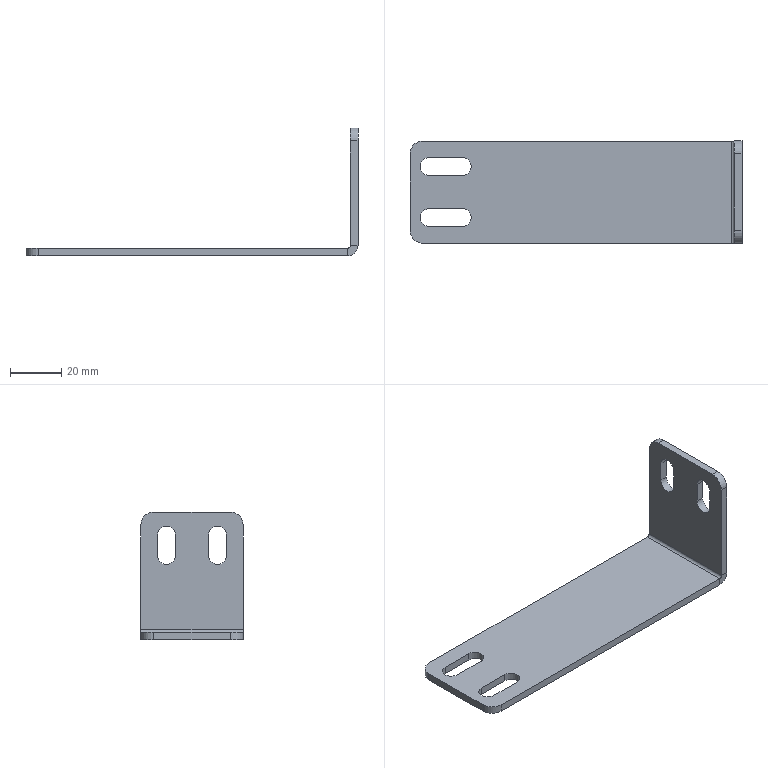Part | STEP file | PN_0061 L-type guardrail connecting plate 130X50_Default<As Machined> | 1 solid | 34 faces | box 130 x 40 x 50 mm | volume 19703 mm3 | plane 20 | cylinder 14 | commonest cylinder face diameters 7 x8 10 x4 2 x1 8 x1